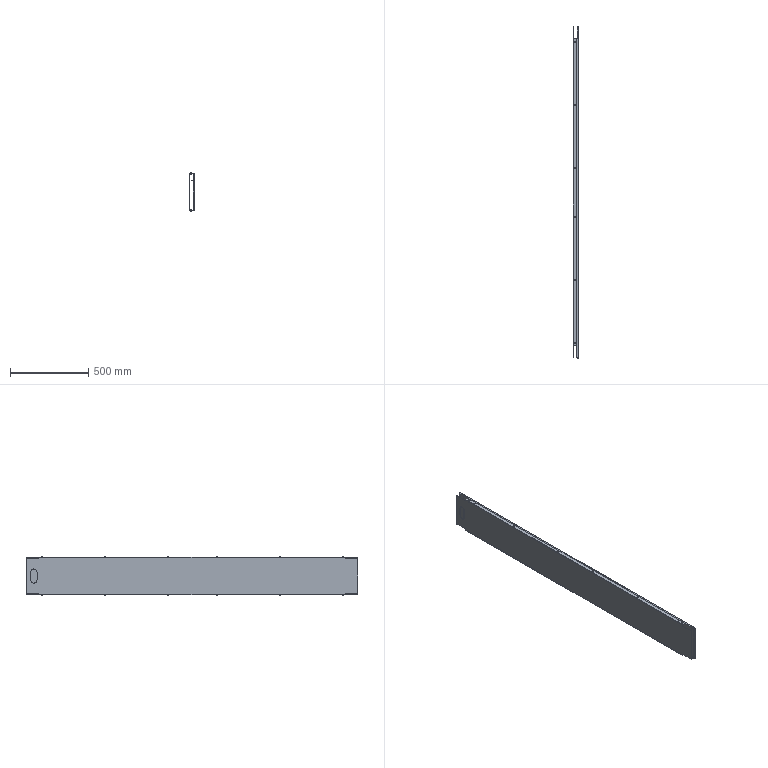Part | SolidWorks | features ReferencePattern 8, MirrorCompFeat 3 | 17 solids | 334 faces | box 36 x 2116 x 253 mm | volume 1688064 mm3 | plane 182 | cylinder 152 | commonest cylinder face diameters 6 x32 6.2 x24 8 x24 8.2 x24 12 x24 7 x9